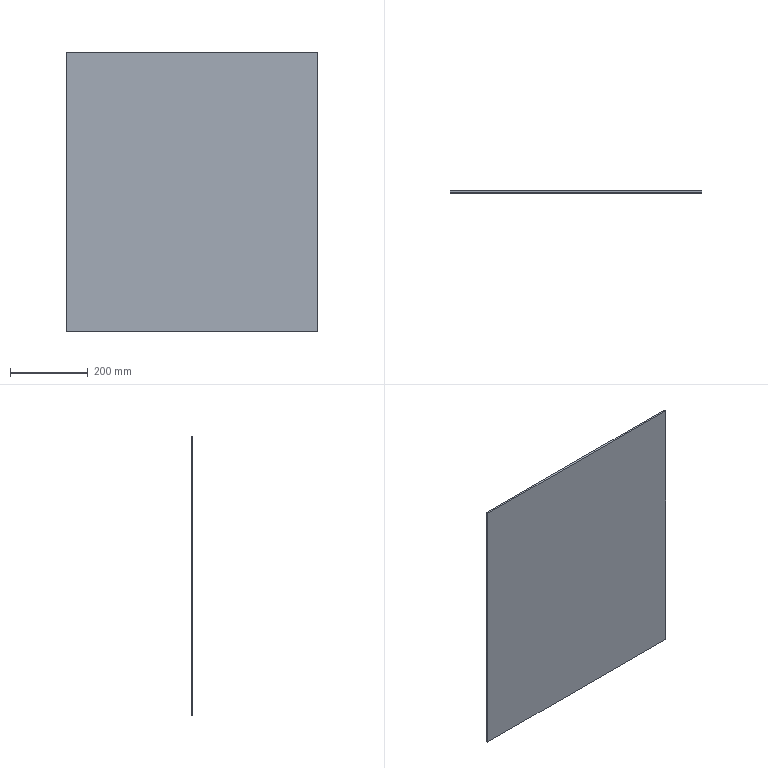Part | SolidWorks | features BaseBody 1, ICE 1 | 1 solid | 6 faces | box 647 x 5 x 720 mm | volume 2329200 mm3 | plane 6
STEP:
#1=CARTESIAN_POINT('',(87.,1835.,360.));
#2=VERTEX_POINT('',#1);
#3=CARTESIAN_POINT('',(87.,1835.,-360.));
#4=VERTEX_POINT('',#3);
#5=CARTESIAN_POINT('',(87.,1835.,0.));
#6=DIRECTION('',(0.,0.,-1.));
#7=VECTOR('',#6,1000.);
#8=LINE('',#5,#7);
#9=EDGE_CURVE('',#2,#4,#8,.T.);
#10=ORIENTED_EDGE('',*,*,#9,.F.);
#11=CARTESIAN_POINT('',(-560.,1835.,360.));
#12=VERTEX_POINT('',#11);
#13=CARTESIAN_POINT('',(-560.,1835.,360.));
#14=DIRECTION('',(1.,0.,0.));
#15=VECTOR('',#14,1000.);
#16=LINE('',#13,#15);
#17=EDGE_CURVE('',#12,#2,#16,.T.);
#18=ORIENTED_EDGE('',*,*,#17,.F.);
#19=CARTESIAN_POINT('',(-560.,1835.,-360.));
#20=VERTEX_POINT('',#19);
#21=CARTESIAN_POINT('',(-560.,1835.,-360.));
#22=DIRECTION('',(0.,0.,1.));
#23=VECTOR('',#22,1000.);
#24=LINE('',#21,#23);
#25=EDGE_CURVE('',#20,#12,#24,.T.);
#26=ORIENTED_EDGE('',*,*,#25,.F.);
#27=CARTESIAN_POINT('',(560.,1835.,-360.));
#28=DIRECTION('',(-1.,0.,0.));
#29=VECTOR('',#28,1000.);
#30=LINE('',#27,#29);
#31=EDGE_CURVE('',#4,#20,#30,.T.);
#32=ORIENTED_EDGE('',*,*,#31,.F.);
#33=EDGE_LOOP('',(#10,#18,#26,#32));
#34=FACE_OUTER_BOUND('',#33,.T.);
#35=CARTESIAN_POINT('',(0.,1835.,0.));
#36=DIRECTION('',(0.,-1.,0.));
#37=DIRECTION('',(0.,0.,-1.));
#38=AXIS2_PLACEMENT_3D('',#35,#36,#37);
#39=PLANE('',#38);
#40=ADVANCED_FACE('',(#34),#39,.T.);
#41=CARTESIAN_POINT('',(87.,1840.,-360.));
#42=VERTEX_POINT('',#41);
#43=CARTESIAN_POINT('',(87.,1840.,360.));
#44=VERTEX_POINT('',#43);
#45=CARTESIAN_POINT('',(87.,1840.,-360.));
#46=DIRECTION('',(0.,0.,1.));
#47=VECTOR('',#46,1000.);
#48=LINE('',#45,#47);
#49=EDGE_CURVE('',#42,#44,#48,.T.);
#50=ORIENTED_EDGE('',*,*,#49,.F.);
#51=CARTESIAN_POINT('',(-560.,1840.,-360.));
#52=VERTEX_POINT('',#51);
#53=CARTESIAN_POINT('',(-560.,1840.,-360.));
#54=DIRECTION('',(1.,0.,0.));
#55=VECTOR('',#54,1000.);
#56=LINE('',#53,#55);
#57=EDGE_CURVE('',#52,#42,#56,.T.);
#58=ORIENTED_EDGE('',*,*,#57,.F.);
#59=CARTESIAN_POINT('',(-560.,1840.,360.));
#60=VERTEX_POINT('',#59);
#61=CARTESIAN_POINT('',(-560.,1840.,360.));
#62=DIRECTION('',(0.,0.,-1.));
#63=VECTOR('',#62,1000.);
#64=LINE('',#61,#63);
#65=EDGE_CURVE('',#60,#52,#64,.T.);
#66=ORIENTED_EDGE('',*,*,#65,.F.);
#67=CARTESIAN_POINT('',(560.,1840.,360.));
#68=DIRECTION('',(-1.,0.,0.));
#69=VECTOR('',#68,1000.);
#70=LINE('',#67,#69);
#71=EDGE_CURVE('',#44,#60,#70,.T.);
#72=ORIENTED_EDGE('',*,*,#71,.F.);
#73=EDGE_LOOP('',(#50,#58,#66,#72));
#74=FACE_OUTER_BOUND('',#73,.T.);
#75=CARTESIAN_POINT('',(0.,1840.,0.));
#76=DIRECTION('',(0.,1.,0.));
#77=DIRECTION('',(1.,0.,0.));
#78=AXIS2_PLACEMENT_3D('',#75,#76,#77);
#79=PLANE('',#78);
#80=ADVANCED_FACE('',(#74),#79,.T.);
#81=ORIENTED_EDGE('',*,*,#65,.T.);
#82=CARTESIAN_POINT('',(-560.,1835.,-360.));
#83=DIRECTION('',(0.,1.,0.));
#84=VECTOR('',#83,1000.);
#85=LINE('',#82,#84);
#86=EDGE_CURVE('',#20,#52,#85,.T.);
#87=ORIENTED_EDGE('',*,*,#86,.F.);
#88=ORIENTED_EDGE('',*,*,#25,.T.);
#89=CARTESIAN_POINT('',(-560.,1840.,360.));
#90=DIRECTION('',(0.,-1.,0.));
#91=VECTOR('',#90,1000.);
#92=LINE('',#89,#91);
#93=EDGE_CURVE('',#60,#12,#92,.T.);
#94=ORIENTED_EDGE('',*,*,#93,.F.);
#95=EDGE_LOOP('',(#81,#87,#88,#94));
#96=FACE_OUTER_BOUND('',#95,.T.);
#97=CARTESIAN_POINT('',(-560.,1840.,360.));
#98=DIRECTION('',(-1.,0.,0.));
#99=DIRECTION('',(0.,0.,1.));
#100=AXIS2_PLACEMENT_3D('',#97,#98,#99);
#101=PLANE('',#100);
#102=ADVANCED_FACE('',(#96),#101,.T.);
#103=CARTESIAN_POINT('',(87.,1830.,-360.));
#104=DIRECTION('',(0.,1.,0.));
#105=VECTOR('',#104,1000.);
#106=LINE('',#103,#105);
#107=EDGE_CURVE('',#4,#42,#106,.T.);
#108=ORIENTED_EDGE('',*,*,#107,.F.);
#109=ORIENTED_EDGE('',*,*,#31,.T.);
#110=ORIENTED_EDGE('',*,*,#86,.T.);
#111=ORIENTED_EDGE('',*,*,#57,.T.);
#112=EDGE_LOOP('',(#108,#109,#110,#111));
#113=FACE_OUTER_BOUND('',#112,.T.);
#114=CARTESIAN_POINT('',(-560.,1840.,-360.));
#115=DIRECTION('',(0.,0.,-1.));
#116=DIRECTION('',(0.,-1.,0.));
#117=AXIS2_PLACEMENT_3D('',#114,#115,#116);
#118=PLANE('',#117);
#119=ADVANCED_FACE('',(#113),#118,.T.);
#120=CARTESIAN_POINT('',(87.,1840.,360.));
#121=DIRECTION('',(0.,-1.,0.));
#122=VECTOR('',#121,1000.);
#123=LINE('',#120,#122);
#124=EDGE_CURVE('',#44,#2,#123,.T.);
#125=ORIENTED_EDGE('',*,*,#124,.F.);
#126=ORIENTED_EDGE('',*,*,#71,.T.);
#127=ORIENTED_EDGE('',*,*,#93,.T.);
#128=ORIENTED_EDGE('',*,*,#17,.T.);
#129=EDGE_LOOP('',(#125,#126,#127,#128));
#130=FACE_OUTER_BOUND('',#129,.T.);
#131=CARTESIAN_POINT('',(560.,1840.,360.));
#132=DIRECTION('',(0.,0.,1.));
#133=DIRECTION('',(1.,0.,0.));
#134=AXIS2_PLACEMENT_3D('',#131,#132,#133);
#135=PLANE('',#134);
#136=ADVANCED_FACE('',(#130),#135,.T.);
#137=ORIENTED_EDGE('',*,*,#9,.T.);
#138=ORIENTED_EDGE('',*,*,#107,.T.);
#139=ORIENTED_EDGE('',*,*,#49,.T.);
#140=ORIENTED_EDGE('',*,*,#124,.T.);
#141=EDGE_LOOP('',(#137,#138,#139,#140));
#142=FACE_OUTER_BOUND('',#141,.T.);
#143=CARTESIAN_POINT('',(87.,1830.,-360.));
#144=DIRECTION('',(-1.,0.,0.));
#145=DIRECTION('',(0.,0.,1.));
#146=AXIS2_PLACEMENT_3D('',#143,#144,#145);
#147=PLANE('',#146);
#148=ADVANCED_FACE('',(#142),#147,.F.);
#149=CLOSED_SHELL('',(#40,#80,#102,#119,#136,#148));
#150=MANIFOLD_SOLID_BREP('',#149);
#151=CARTESIAN_POINT('',(0.,0.,0.));
#152=DIRECTION('',(0.,0.,1.));
#153=DIRECTION('',(1.,0.,0.));
#154=AXIS2_PLACEMENT_3D('',#151,#152,#153);
#155=(LENGTH_UNIT()NAMED_UNIT(*)SI_UNIT(.MILLI.,.METRE.));
#156=UNCERTAINTY_MEASURE_WITH_UNIT(LENGTH_MEASURE(0.00001),#155,'','');
#157=(NAMED_UNIT(*)PLANE_ANGLE_UNIT()SI_UNIT($,.RADIAN.));
#158=(NAMED_UNIT(*)SI_UNIT($,.STERADIAN.)SOLID_ANGLE_UNIT());
#159=(GEOMETRIC_REPRESENTATION_CONTEXT(3)GLOBAL_UNCERTAINTY_ASSIGNED_CONTEXT((#156))GLOBAL_UNIT_ASSIGNED_CONTEXT((#155,#157,#158))REPRESENTATION_CONTEXT('',''));
#160=ADVANCED_BREP_SHAPE_REPRESENTATION('',(#150,#154),#159);